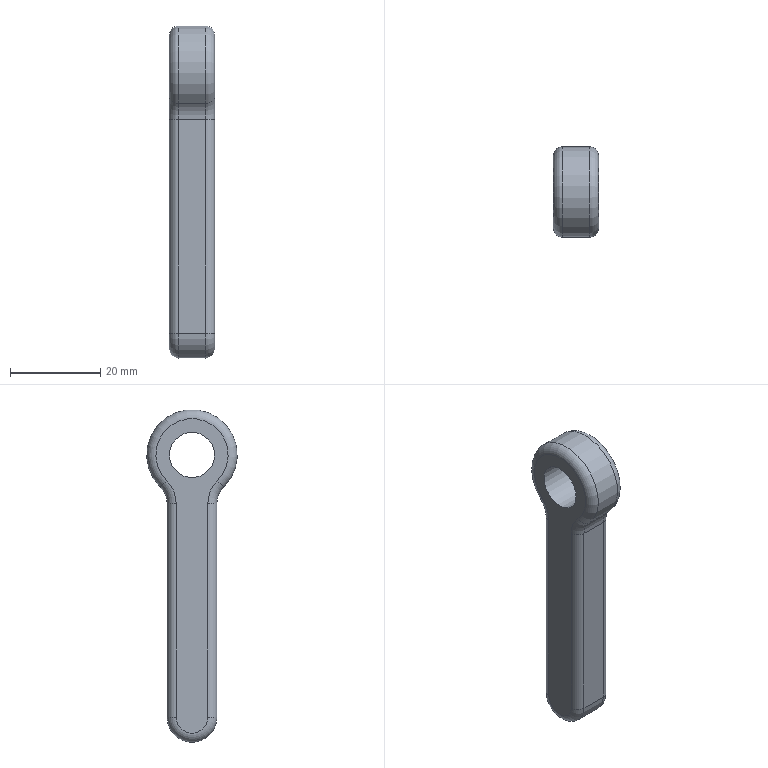Part | NX | features DATUM_CSYS 2, BLEND 1, EXTRUDE 1, SKETCH 1 | 1 solid | 21 faces | box 10 x 20 x 73.5 mm | volume 7901 mm3 | cylinder 9 | torus 8 | plane 4 | commonest cylinder face diameters 4 x4 10 x3 11 x1 20 x1
STEP:
#1=CARTESIAN_POINT('',(8.,-7.,-7.141));
#2=VERTEX_POINT('',#1);
#3=CARTESIAN_POINT('',(2.,-7.,-7.141));
#4=VERTEX_POINT('',#3);
#5=CARTESIAN_POINT('',(10.,-7.,-7.141));
#6=DIRECTION('',(-1.,0.,0.));
#7=VECTOR('',#6,1000.);
#8=LINE('',#5,#7);
#9=EDGE_CURVE('',#2,#4,#8,.T.);
#10=ORIENTED_EDGE('',*,*,#9,.T.);
#11=CARTESIAN_POINT('',(2.,-5.5,-10.712));
#12=VERTEX_POINT('',#11);
#13=CARTESIAN_POINT('',(2.,-10.5,-10.712));
#14=DIRECTION('',(-1.,0.,0.));
#15=DIRECTION('',(0.,0.,1.));
#16=AXIS2_PLACEMENT_3D('',#13,#14,#15);
#17=CIRCLE('',#16,5.);
#18=EDGE_CURVE('',#4,#12,#17,.T.);
#19=ORIENTED_EDGE('',*,*,#18,.T.);
#20=CARTESIAN_POINT('',(8.,-5.5,-10.712));
#21=VERTEX_POINT('',#20);
#22=CARTESIAN_POINT('',(10.,-5.5,-10.712));
#23=DIRECTION('',(-1.,0.,0.));
#24=VECTOR('',#23,1000.);
#25=LINE('',#22,#24);
#26=EDGE_CURVE('',#21,#12,#25,.T.);
#27=ORIENTED_EDGE('',*,*,#26,.F.);
#28=CARTESIAN_POINT('',(8.,-10.5,-10.712));
#29=DIRECTION('',(-1.,0.,0.));
#30=DIRECTION('',(0.,0.,1.));
#31=AXIS2_PLACEMENT_3D('',#28,#29,#30);
#32=CIRCLE('',#31,5.);
#33=EDGE_CURVE('',#21,#2,#32,.F.);
#34=ORIENTED_EDGE('',*,*,#33,.T.);
#35=EDGE_LOOP('',(#10,#19,#27,#34));
#36=FACE_BOUND('',#35,.T.);
#37=CARTESIAN_POINT('',(10.,-10.5,-10.712));
#38=DIRECTION('',(-1.,0.,0.));
#39=DIRECTION('',(0.,0.,1.));
#40=AXIS2_PLACEMENT_3D('',#37,#38,#39);
#41=CYLINDRICAL_SURFACE('',#40,5.);
#42=ADVANCED_FACE('',(#36),#41,.F.);
#43=ORIENTED_EDGE('',*,*,#26,.T.);
#44=CARTESIAN_POINT('',(2.,-5.5,-58.));
#45=VERTEX_POINT('',#44);
#46=CARTESIAN_POINT('',(2.,-5.5,-58.));
#47=DIRECTION('',(0.,0.,-1.));
#48=VECTOR('',#47,1000.);
#49=LINE('',#46,#48);
#50=EDGE_CURVE('',#12,#45,#49,.T.);
#51=ORIENTED_EDGE('',*,*,#50,.T.);
#52=CARTESIAN_POINT('',(8.,-5.5,-58.));
#53=VERTEX_POINT('',#52);
#54=CARTESIAN_POINT('',(10.,-5.5,-58.));
#55=DIRECTION('',(-1.,0.,0.));
#56=VECTOR('',#55,1000.);
#57=LINE('',#54,#56);
#58=EDGE_CURVE('',#53,#45,#57,.T.);
#59=ORIENTED_EDGE('',*,*,#58,.F.);
#60=CARTESIAN_POINT('',(8.,-5.5,-10.712));
#61=DIRECTION('',(0.,0.,-1.));
#62=VECTOR('',#61,1000.);
#63=LINE('',#60,#62);
#64=EDGE_CURVE('',#53,#21,#63,.F.);
#65=ORIENTED_EDGE('',*,*,#64,.T.);
#66=EDGE_LOOP('',(#43,#51,#59,#65));
#67=FACE_BOUND('',#66,.T.);
#68=CARTESIAN_POINT('',(10.,-5.5,-10.712));
#69=DIRECTION('',(0.,1.,0.));
#70=DIRECTION('',(0.,0.,1.));
#71=AXIS2_PLACEMENT_3D('',#68,#69,#70);
#72=PLANE('',#71);
#73=ADVANCED_FACE('',(#67),#72,.F.);
#74=ORIENTED_EDGE('',*,*,#58,.T.);
#75=CARTESIAN_POINT('',(2.,5.5,-58.));
#76=VERTEX_POINT('',#75);
#77=CARTESIAN_POINT('',(2.,0.,-58.));
#78=DIRECTION('',(-1.,0.,0.));
#79=DIRECTION('',(0.,0.,1.));
#80=AXIS2_PLACEMENT_3D('',#77,#78,#79);
#81=CIRCLE('',#80,5.5);
#82=EDGE_CURVE('',#45,#76,#81,.F.);
#83=ORIENTED_EDGE('',*,*,#82,.T.);
#84=CARTESIAN_POINT('',(8.,5.5,-58.));
#85=VERTEX_POINT('',#84);
#86=CARTESIAN_POINT('',(10.,5.5,-58.));
#87=DIRECTION('',(-1.,0.,0.));
#88=VECTOR('',#87,1000.);
#89=LINE('',#86,#88);
#90=EDGE_CURVE('',#85,#76,#89,.T.);
#91=ORIENTED_EDGE('',*,*,#90,.F.);
#92=CARTESIAN_POINT('',(8.,0.,-58.));
#93=DIRECTION('',(-1.,0.,0.));
#94=DIRECTION('',(0.,0.,1.));
#95=AXIS2_PLACEMENT_3D('',#92,#93,#94);
#96=CIRCLE('',#95,5.5);
#97=EDGE_CURVE('',#85,#53,#96,.T.);
#98=ORIENTED_EDGE('',*,*,#97,.T.);
#99=EDGE_LOOP('',(#74,#83,#91,#98));
#100=FACE_BOUND('',#99,.T.);
#101=CARTESIAN_POINT('',(10.,0.,-58.));
#102=DIRECTION('',(-1.,0.,0.));
#103=DIRECTION('',(0.,0.,1.));
#104=AXIS2_PLACEMENT_3D('',#101,#102,#103);
#105=CYLINDRICAL_SURFACE('',#104,5.5);
#106=ADVANCED_FACE('',(#100),#105,.T.);
#107=ORIENTED_EDGE('',*,*,#90,.T.);
#108=CARTESIAN_POINT('',(2.,5.5,-10.712));
#109=VERTEX_POINT('',#108);
#110=CARTESIAN_POINT('',(2.,5.5,-10.712));
#111=DIRECTION('',(0.,0.,1.));
#112=VECTOR('',#111,1000.);
#113=LINE('',#110,#112);
#114=EDGE_CURVE('',#76,#109,#113,.T.);
#115=ORIENTED_EDGE('',*,*,#114,.T.);
#116=CARTESIAN_POINT('',(8.,5.5,-10.712));
#117=VERTEX_POINT('',#116);
#118=CARTESIAN_POINT('',(10.,5.5,-10.712));
#119=DIRECTION('',(-1.,0.,0.));
#120=VECTOR('',#119,1000.);
#121=LINE('',#118,#120);
#122=EDGE_CURVE('',#117,#109,#121,.T.);
#123=ORIENTED_EDGE('',*,*,#122,.F.);
#124=CARTESIAN_POINT('',(8.,5.5,-58.));
#125=DIRECTION('',(0.,0.,1.));
#126=VECTOR('',#125,1000.);
#127=LINE('',#124,#126);
#128=EDGE_CURVE('',#117,#85,#127,.F.);
#129=ORIENTED_EDGE('',*,*,#128,.T.);
#130=EDGE_LOOP('',(#107,#115,#123,#129));
#131=FACE_BOUND('',#130,.T.);
#132=CARTESIAN_POINT('',(10.,5.5,-58.));
#133=DIRECTION('',(0.,-1.,0.));
#134=DIRECTION('',(0.,0.,-1.));
#135=AXIS2_PLACEMENT_3D('',#132,#133,#134);
#136=PLANE('',#135);
#137=ADVANCED_FACE('',(#131),#136,.F.);
#138=ORIENTED_EDGE('',*,*,#122,.T.);
#139=CARTESIAN_POINT('',(2.,7.,-7.141));
#140=VERTEX_POINT('',#139);
#141=CARTESIAN_POINT('',(2.,10.5,-10.712));
#142=DIRECTION('',(-1.,0.,0.));
#143=DIRECTION('',(0.,0.,1.));
#144=AXIS2_PLACEMENT_3D('',#141,#142,#143);
#145=CIRCLE('',#144,5.);
#146=EDGE_CURVE('',#109,#140,#145,.T.);
#147=ORIENTED_EDGE('',*,*,#146,.T.);
#148=CARTESIAN_POINT('',(8.,7.,-7.141));
#149=VERTEX_POINT('',#148);
#150=CARTESIAN_POINT('',(10.,7.,-7.141));
#151=DIRECTION('',(-1.,0.,0.));
#152=VECTOR('',#151,1000.);
#153=LINE('',#150,#152);
#154=EDGE_CURVE('',#149,#140,#153,.T.);
#155=ORIENTED_EDGE('',*,*,#154,.F.);
#156=CARTESIAN_POINT('',(8.,10.5,-10.712));
#157=DIRECTION('',(-1.,0.,0.));
#158=DIRECTION('',(0.,0.,1.));
#159=AXIS2_PLACEMENT_3D('',#156,#157,#158);
#160=CIRCLE('',#159,5.);
#161=EDGE_CURVE('',#149,#117,#160,.F.);
#162=ORIENTED_EDGE('',*,*,#161,.T.);
#163=EDGE_LOOP('',(#138,#147,#155,#162));
#164=FACE_BOUND('',#163,.T.);
#165=CARTESIAN_POINT('',(10.,10.5,-10.712));
#166=DIRECTION('',(-1.,0.,0.));
#167=DIRECTION('',(0.,0.,1.));
#168=AXIS2_PLACEMENT_3D('',#165,#166,#167);
#169=CYLINDRICAL_SURFACE('',#168,5.);
#170=ADVANCED_FACE('',(#164),#169,.F.);
#171=ORIENTED_EDGE('',*,*,#154,.T.);
#172=CARTESIAN_POINT('',(2.,0.,0.));
#173=DIRECTION('',(-1.,0.,0.));
#174=DIRECTION('',(0.,0.,1.));
#175=AXIS2_PLACEMENT_3D('',#172,#173,#174);
#176=CIRCLE('',#175,10.);
#177=EDGE_CURVE('',#140,#4,#176,.F.);
#178=ORIENTED_EDGE('',*,*,#177,.T.);
#179=ORIENTED_EDGE('',*,*,#9,.F.);
#180=CARTESIAN_POINT('',(8.,0.,0.));
#181=DIRECTION('',(-1.,0.,0.));
#182=DIRECTION('',(0.,0.,1.));
#183=AXIS2_PLACEMENT_3D('',#180,#181,#182);
#184=CIRCLE('',#183,10.);
#185=EDGE_CURVE('',#2,#149,#184,.T.);
#186=ORIENTED_EDGE('',*,*,#185,.T.);
#187=EDGE_LOOP('',(#171,#178,#179,#186));
#188=FACE_BOUND('',#187,.T.);
#189=CARTESIAN_POINT('',(10.,0.,0.));
#190=DIRECTION('',(-1.,0.,0.));
#191=DIRECTION('',(0.,0.,1.));
#192=AXIS2_PLACEMENT_3D('',#189,#190,#191);
#193=CYLINDRICAL_SURFACE('',#192,10.);
#194=ADVANCED_FACE('',(#188),#193,.T.);
#195=CARTESIAN_POINT('',(10.,5.,0.));
#196=VERTEX_POINT('',#195);
#197=CARTESIAN_POINT('',(10.,0.,0.));
#198=DIRECTION('',(1.,0.,0.));
#199=DIRECTION('',(0.,1.,0.));
#200=AXIS2_PLACEMENT_3D('',#197,#198,#199);
#201=CIRCLE('',#200,5.);
#202=EDGE_CURVE('',#196,#196,#201,.T.);
#203=ORIENTED_EDGE('',*,*,#202,.T.);
#204=EDGE_LOOP('',(#203));
#205=FACE_BOUND('',#204,.T.);
#206=CARTESIAN_POINT('',(0.,5.,0.));
#207=VERTEX_POINT('',#206);
#208=CARTESIAN_POINT('',(0.,0.,0.));
#209=DIRECTION('',(1.,0.,0.));
#210=DIRECTION('',(0.,1.,0.));
#211=AXIS2_PLACEMENT_3D('',#208,#209,#210);
#212=CIRCLE('',#211,5.);
#213=EDGE_CURVE('',#207,#207,#212,.T.);
#214=ORIENTED_EDGE('',*,*,#213,.F.);
#215=EDGE_LOOP('',(#214));
#216=FACE_BOUND('',#215,.T.);
#217=CARTESIAN_POINT('',(10.,0.,0.));
#218=DIRECTION('',(-1.,0.,0.));
#219=DIRECTION('',(0.,0.,1.));
#220=AXIS2_PLACEMENT_3D('',#217,#218,#219);
#221=CYLINDRICAL_SURFACE('',#220,5.);
#222=ADVANCED_FACE('',(#205,#216),#221,.F.);
#223=CARTESIAN_POINT('',(10.,3.5,-58.));
#224=VERTEX_POINT('',#223);
#225=CARTESIAN_POINT('',(10.,3.5,-10.712));
#226=VERTEX_POINT('',#225);
#227=CARTESIAN_POINT('',(10.,3.5,-10.712));
#228=DIRECTION('',(0.,0.,1.));
#229=VECTOR('',#228,1000.);
#230=LINE('',#227,#229);
#231=EDGE_CURVE('',#224,#226,#230,.T.);
#232=ORIENTED_EDGE('',*,*,#231,.T.);
#233=CARTESIAN_POINT('',(10.,5.6,-5.713));
#234=VERTEX_POINT('',#233);
#235=CARTESIAN_POINT('',(10.,10.5,-10.712));
#236=DIRECTION('',(-1.,0.,0.));
#237=DIRECTION('',(0.,0.,1.));
#238=AXIS2_PLACEMENT_3D('',#235,#236,#237);
#239=CIRCLE('',#238,7.);
#240=EDGE_CURVE('',#226,#234,#239,.T.);
#241=ORIENTED_EDGE('',*,*,#240,.T.);
#242=CARTESIAN_POINT('',(10.,-5.6,-5.713));
#243=VERTEX_POINT('',#242);
#244=CARTESIAN_POINT('',(10.,0.,0.));
#245=DIRECTION('',(-1.,0.,0.));
#246=DIRECTION('',(0.,0.,1.));
#247=AXIS2_PLACEMENT_3D('',#244,#245,#246);
#248=CIRCLE('',#247,8.);
#249=EDGE_CURVE('',#234,#243,#248,.F.);
#250=ORIENTED_EDGE('',*,*,#249,.T.);
#251=CARTESIAN_POINT('',(10.,-3.5,-10.712));
#252=VERTEX_POINT('',#251);
#253=CARTESIAN_POINT('',(10.,-10.5,-10.712));
#254=DIRECTION('',(-1.,0.,0.));
#255=DIRECTION('',(0.,0.,1.));
#256=AXIS2_PLACEMENT_3D('',#253,#254,#255);
#257=CIRCLE('',#256,7.);
#258=EDGE_CURVE('',#243,#252,#257,.T.);
#259=ORIENTED_EDGE('',*,*,#258,.T.);
#260=CARTESIAN_POINT('',(10.,-3.5,-58.));
#261=VERTEX_POINT('',#260);
#262=CARTESIAN_POINT('',(10.,-3.5,-10.712));
#263=DIRECTION('',(0.,0.,-1.));
#264=VECTOR('',#263,1000.);
#265=LINE('',#262,#264);
#266=EDGE_CURVE('',#252,#261,#265,.T.);
#267=ORIENTED_EDGE('',*,*,#266,.T.);
#268=CARTESIAN_POINT('',(10.,0.,-58.));
#269=DIRECTION('',(-1.,0.,0.));
#270=DIRECTION('',(0.,0.,1.));
#271=AXIS2_PLACEMENT_3D('',#268,#269,#270);
#272=CIRCLE('',#271,3.5);
#273=EDGE_CURVE('',#261,#224,#272,.F.);
#274=ORIENTED_EDGE('',*,*,#273,.T.);
#275=EDGE_LOOP('',(#232,#241,#250,#259,#267,#274));
#276=FACE_BOUND('',#275,.T.);
#277=ORIENTED_EDGE('',*,*,#202,.F.);
#278=EDGE_LOOP('',(#277));
#279=FACE_BOUND('',#278,.T.);
#280=CARTESIAN_POINT('',(10.,-10.5,-10.712));
#281=DIRECTION('',(-1.,0.,0.));
#282=DIRECTION('',(0.,0.,1.));
#283=AXIS2_PLACEMENT_3D('',#280,#281,#282);
#284=PLANE('',#283);
#285=ADVANCED_FACE('',(#276,#279),#284,.F.);
#286=CARTESIAN_POINT('',(0.,3.5,-58.));
#287=VERTEX_POINT('',#286);
#288=CARTESIAN_POINT('',(0.,-3.5,-58.));
#289=VERTEX_POINT('',#288);
#290=CARTESIAN_POINT('',(0.,0.,-58.));
#291=DIRECTION('',(-1.,0.,0.));
#292=DIRECTION('',(0.,0.,1.));
#293=AXIS2_PLACEMENT_3D('',#290,#291,#292);
#294=CIRCLE('',#293,3.5);
#295=EDGE_CURVE('',#287,#289,#294,.T.);
#296=ORIENTED_EDGE('',*,*,#295,.T.);
#297=CARTESIAN_POINT('',(0.,-3.5,-10.712));
#298=VERTEX_POINT('',#297);
#299=CARTESIAN_POINT('',(0.,-3.5,-10.712));
#300=DIRECTION('',(0.,0.,-1.));
#301=VECTOR('',#300,1000.);
#302=LINE('',#299,#301);
#303=EDGE_CURVE('',#289,#298,#302,.F.);
#304=ORIENTED_EDGE('',*,*,#303,.T.);
#305=CARTESIAN_POINT('',(0.,-5.6,-5.713));
#306=VERTEX_POINT('',#305);
#307=CARTESIAN_POINT('',(0.,-10.5,-10.712));
#308=DIRECTION('',(-1.,0.,0.));
#309=DIRECTION('',(0.,0.,1.));
#310=AXIS2_PLACEMENT_3D('',#307,#308,#309);
#311=CIRCLE('',#310,7.);
#312=EDGE_CURVE('',#298,#306,#311,.F.);
#313=ORIENTED_EDGE('',*,*,#312,.T.);
#314=CARTESIAN_POINT('',(0.,5.6,-5.713));
#315=VERTEX_POINT('',#314);
#316=CARTESIAN_POINT('',(0.,0.,0.));
#317=DIRECTION('',(-1.,0.,0.));
#318=DIRECTION('',(0.,0.,1.));
#319=AXIS2_PLACEMENT_3D('',#316,#317,#318);
#320=CIRCLE('',#319,8.);
#321=EDGE_CURVE('',#306,#315,#320,.T.);
#322=ORIENTED_EDGE('',*,*,#321,.T.);
#323=CARTESIAN_POINT('',(0.,3.5,-10.712));
#324=VERTEX_POINT('',#323);
#325=CARTESIAN_POINT('',(0.,10.5,-10.712));
#326=DIRECTION('',(-1.,0.,0.));
#327=DIRECTION('',(0.,0.,1.));
#328=AXIS2_PLACEMENT_3D('',#325,#326,#327);
#329=CIRCLE('',#328,7.);
#330=EDGE_CURVE('',#315,#324,#329,.F.);
#331=ORIENTED_EDGE('',*,*,#330,.T.);
#332=CARTESIAN_POINT('',(0.,3.5,-58.));
#333=DIRECTION('',(0.,0.,1.));
#334=VECTOR('',#333,1000.);
#335=LINE('',#332,#334);
#336=EDGE_CURVE('',#324,#287,#335,.F.);
#337=ORIENTED_EDGE('',*,*,#336,.T.);
#338=EDGE_LOOP('',(#296,#304,#313,#322,#331,#337));
#339=FACE_BOUND('',#338,.T.);
#340=ORIENTED_EDGE('',*,*,#213,.T.);
#341=EDGE_LOOP('',(#340));
#342=FACE_BOUND('',#341,.T.);
#343=CARTESIAN_POINT('',(0.,-10.5,-10.712));
#344=DIRECTION('',(-1.,0.,0.));
#345=DIRECTION('',(0.,0.,1.));
#346=AXIS2_PLACEMENT_3D('',#343,#344,#345);
#347=PLANE('',#346);
#348=ADVANCED_FACE('',(#339,#342),#347,.T.);
#349=CARTESIAN_POINT('',(2.,3.5,-10.712));
#350=DIRECTION('',(0.,0.,-1.));
#351=DIRECTION('',(-1.,0.,0.));
#352=AXIS2_PLACEMENT_3D('',#349,#350,#351);
#353=CIRCLE('',#352,2.);
#354=EDGE_CURVE('',#324,#109,#353,.T.);
#355=ORIENTED_EDGE('',*,*,#354,.F.);
#356=ORIENTED_EDGE('',*,*,#330,.F.);
#357=CARTESIAN_POINT('',(2.,5.6,-5.713));
#358=DIRECTION('',(0.,0.7141,0.7));
#359=DIRECTION('',(0.,-0.7,0.7141));
#360=AXIS2_PLACEMENT_3D('',#357,#358,#359);
#361=CIRCLE('',#360,2.);
#362=EDGE_CURVE('',#140,#315,#361,.T.);
#363=ORIENTED_EDGE('',*,*,#362,.F.);
#364=ORIENTED_EDGE('',*,*,#146,.F.);
#365=EDGE_LOOP('',(#355,#356,#363,#364));
#366=FACE_BOUND('',#365,.T.);
#367=CARTESIAN_POINT('',(2.,10.5,-10.712));
#368=DIRECTION('',(-1.,0.,0.));
#369=DIRECTION('',(0.,0.,1.));
#370=AXIS2_PLACEMENT_3D('',#367,#368,#369);
#371=TOROIDAL_SURFACE('',#370,7.,2.);
#372=ADVANCED_FACE('',(#366),#371,.T.);
#373=ORIENTED_EDGE('',*,*,#362,.T.);
#374=ORIENTED_EDGE('',*,*,#321,.F.);
#375=CARTESIAN_POINT('',(2.,-5.6,-5.713));
#376=DIRECTION('',(0.,0.7141,-0.7));
#377=DIRECTION('',(0.,0.7,0.7141));
#378=AXIS2_PLACEMENT_3D('',#375,#376,#377);
#379=CIRCLE('',#378,2.);
#380=EDGE_CURVE('',#4,#306,#379,.T.);
#381=ORIENTED_EDGE('',*,*,#380,.F.);
#382=ORIENTED_EDGE('',*,*,#177,.F.);
#383=EDGE_LOOP('',(#373,#374,#381,#382));
#384=FACE_BOUND('',#383,.T.);
#385=CARTESIAN_POINT('',(2.,0.,0.));
#386=DIRECTION('',(-1.,0.,0.));
#387=DIRECTION('',(0.,0.,1.));
#388=AXIS2_PLACEMENT_3D('',#385,#386,#387);
#389=TOROIDAL_SURFACE('',#388,8.,2.);
#390=ADVANCED_FACE('',(#384),#389,.T.);
#391=ORIENTED_EDGE('',*,*,#354,.T.);
#392=ORIENTED_EDGE('',*,*,#114,.F.);
#393=CARTESIAN_POINT('',(2.,3.5,-58.));
#394=DIRECTION('',(0.,0.,-1.));
#395=DIRECTION('',(-1.,0.,0.));
#396=AXIS2_PLACEMENT_3D('',#393,#394,#395);
#397=CIRCLE('',#396,2.);
#398=EDGE_CURVE('',#287,#76,#397,.T.);
#399=ORIENTED_EDGE('',*,*,#398,.F.);
#400=ORIENTED_EDGE('',*,*,#336,.F.);
#401=EDGE_LOOP('',(#391,#392,#399,#400));
#402=FACE_BOUND('',#401,.T.);
#403=CARTESIAN_POINT('',(2.,3.5,-58.));
#404=DIRECTION('',(0.,0.,-1.));
#405=DIRECTION('',(0.,1.,0.));
#406=AXIS2_PLACEMENT_3D('',#403,#404,#405);
#407=CYLINDRICAL_SURFACE('',#406,2.);
#408=ADVANCED_FACE('',(#402),#407,.T.);
#409=ORIENTED_EDGE('',*,*,#380,.T.);
#410=ORIENTED_EDGE('',*,*,#312,.F.);
#411=CARTESIAN_POINT('',(2.,-3.5,-10.712));
#412=DIRECTION('',(0.,0.,-1.));
#413=DIRECTION('',(-1.,0.,0.));
#414=AXIS2_PLACEMENT_3D('',#411,#412,#413);
#415=CIRCLE('',#414,2.);
#416=EDGE_CURVE('',#12,#298,#415,.T.);
#417=ORIENTED_EDGE('',*,*,#416,.F.);
#418=ORIENTED_EDGE('',*,*,#18,.F.);
#419=EDGE_LOOP('',(#409,#410,#417,#418));
#420=FACE_BOUND('',#419,.T.);
#421=CARTESIAN_POINT('',(2.,-10.5,-10.712));
#422=DIRECTION('',(-1.,0.,0.));
#423=DIRECTION('',(0.,0.,1.));
#424=AXIS2_PLACEMENT_3D('',#421,#422,#423);
#425=TOROIDAL_SURFACE('',#424,7.,2.);
#426=ADVANCED_FACE('',(#420),#425,.T.);
#427=ORIENTED_EDGE('',*,*,#398,.T.);
#428=ORIENTED_EDGE('',*,*,#82,.F.);
#429=CARTESIAN_POINT('',(2.,-3.5,-58.));
#430=DIRECTION('',(0.,0.,1.));
#431=DIRECTION('',(1.,0.,0.));
#432=AXIS2_PLACEMENT_3D('',#429,#430,#431);
#433=CIRCLE('',#432,2.);
#434=EDGE_CURVE('',#289,#45,#433,.T.);
#435=ORIENTED_EDGE('',*,*,#434,.F.);
#436=ORIENTED_EDGE('',*,*,#295,.F.);
#437=EDGE_LOOP('',(#427,#428,#435,#436));
#438=FACE_BOUND('',#437,.T.);
#439=CARTESIAN_POINT('',(2.,0.,-58.));
#440=DIRECTION('',(-1.,0.,0.));
#441=DIRECTION('',(0.,0.,1.));
#442=AXIS2_PLACEMENT_3D('',#439,#440,#441);
#443=TOROIDAL_SURFACE('',#442,3.5,2.);
#444=ADVANCED_FACE('',(#438),#443,.T.);
#445=ORIENTED_EDGE('',*,*,#416,.T.);
#446=ORIENTED_EDGE('',*,*,#303,.F.);
#447=ORIENTED_EDGE('',*,*,#434,.T.);
#448=ORIENTED_EDGE('',*,*,#50,.F.);
#449=EDGE_LOOP('',(#445,#446,#447,#448));
#450=FACE_BOUND('',#449,.T.);
#451=CARTESIAN_POINT('',(2.,-3.5,-10.712));
#452=DIRECTION('',(0.,0.,1.));
#453=DIRECTION('',(0.,-1.,0.));
#454=AXIS2_PLACEMENT_3D('',#451,#452,#453);
#455=CYLINDRICAL_SURFACE('',#454,2.);
#456=ADVANCED_FACE('',(#450),#455,.T.);
#457=CARTESIAN_POINT('',(8.,-3.5,-10.712));
#458=DIRECTION('',(0.,0.,1.));
#459=DIRECTION('',(1.,0.,0.));
#460=AXIS2_PLACEMENT_3D('',#457,#458,#459);
#461=CIRCLE('',#460,2.);
#462=EDGE_CURVE('',#21,#252,#461,.T.);
#463=ORIENTED_EDGE('',*,*,#462,.F.);
#464=ORIENTED_EDGE('',*,*,#64,.F.);
#465=CARTESIAN_POINT('',(8.,-3.5,-58.));
#466=DIRECTION('',(0.,0.,-1.));
#467=DIRECTION('',(-1.,0.,0.));
#468=AXIS2_PLACEMENT_3D('',#465,#466,#467);
#469=CIRCLE('',#468,2.);
#470=EDGE_CURVE('',#261,#53,#469,.T.);
#471=ORIENTED_EDGE('',*,*,#470,.F.);
#472=ORIENTED_EDGE('',*,*,#266,.F.);
#473=EDGE_LOOP('',(#463,#464,#471,#472));
#474=FACE_BOUND('',#473,.T.);
#475=CARTESIAN_POINT('',(8.,-3.5,-10.712));
#476=DIRECTION('',(0.,0.,-1.));
#477=DIRECTION('',(0.,1.,0.));
#478=AXIS2_PLACEMENT_3D('',#475,#476,#477);
#479=CYLINDRICAL_SURFACE('',#478,2.);
#480=ADVANCED_FACE('',(#474),#479,.T.);
#481=ORIENTED_EDGE('',*,*,#470,.T.);
#482=ORIENTED_EDGE('',*,*,#97,.F.);
#483=CARTESIAN_POINT('',(8.,3.5,-58.));
#484=DIRECTION('',(0.,0.,1.));
#485=DIRECTION('',(1.,0.,0.));
#486=AXIS2_PLACEMENT_3D('',#483,#484,#485);
#487=CIRCLE('',#486,2.);
#488=EDGE_CURVE('',#224,#85,#487,.T.);
#489=ORIENTED_EDGE('',*,*,#488,.F.);
#490=ORIENTED_EDGE('',*,*,#273,.F.);
#491=EDGE_LOOP('',(#481,#482,#489,#490));
#492=FACE_BOUND('',#491,.T.);
#493=CARTESIAN_POINT('',(8.,0.,-58.));
#494=DIRECTION('',(-1.,0.,0.));
#495=DIRECTION('',(0.,0.,1.));
#496=AXIS2_PLACEMENT_3D('',#493,#494,#495);
#497=TOROIDAL_SURFACE('',#496,3.5,2.);
#498=ADVANCED_FACE('',(#492),#497,.T.);
#499=ORIENTED_EDGE('',*,*,#462,.T.);
#500=ORIENTED_EDGE('',*,*,#258,.F.);
#501=CARTESIAN_POINT('',(8.,-5.6,-5.713));
#502=DIRECTION('',(0.,-0.7141,0.7));
#503=DIRECTION('',(0.,-0.7,-0.7141));
#504=AXIS2_PLACEMENT_3D('',#501,#502,#503);
#505=CIRCLE('',#504,2.);
#506=EDGE_CURVE('',#2,#243,#505,.T.);
#507=ORIENTED_EDGE('',*,*,#506,.F.);
#508=ORIENTED_EDGE('',*,*,#33,.F.);
#509=EDGE_LOOP('',(#499,#500,#507,#508));
#510=FACE_BOUND('',#509,.T.);
#511=CARTESIAN_POINT('',(8.,-10.5,-10.712));
#512=DIRECTION('',(-1.,0.,0.));
#513=DIRECTION('',(0.,0.,1.));
#514=AXIS2_PLACEMENT_3D('',#511,#512,#513);
#515=TOROIDAL_SURFACE('',#514,7.,2.);
#516=ADVANCED_FACE('',(#510),#515,.T.);
#517=ORIENTED_EDGE('',*,*,#488,.T.);
#518=ORIENTED_EDGE('',*,*,#128,.F.);
#519=CARTESIAN_POINT('',(8.,3.5,-10.712));
#520=DIRECTION('',(0.,0.,1.));
#521=DIRECTION('',(1.,0.,0.));
#522=AXIS2_PLACEMENT_3D('',#519,#520,#521);
#523=CIRCLE('',#522,2.);
#524=EDGE_CURVE('',#226,#117,#523,.T.);
#525=ORIENTED_EDGE('',*,*,#524,.F.);
#526=ORIENTED_EDGE('',*,*,#231,.F.);
#527=EDGE_LOOP('',(#517,#518,#525,#526));
#528=FACE_BOUND('',#527,.T.);
#529=CARTESIAN_POINT('',(8.,3.5,-10.712));
#530=DIRECTION('',(0.,0.,1.));
#531=DIRECTION('',(0.,-1.,0.));
#532=AXIS2_PLACEMENT_3D('',#529,#530,#531);
#533=CYLINDRICAL_SURFACE('',#532,2.);
#534=ADVANCED_FACE('',(#528),#533,.T.);
#535=ORIENTED_EDGE('',*,*,#506,.T.);
#536=ORIENTED_EDGE('',*,*,#249,.F.);
#537=CARTESIAN_POINT('',(8.,5.6,-5.713));
#538=DIRECTION('',(0.,-0.7141,-0.7));
#539=DIRECTION('',(0.,0.7,-0.7141));
#540=AXIS2_PLACEMENT_3D('',#537,#538,#539);
#541=CIRCLE('',#540,2.);
#542=EDGE_CURVE('',#149,#234,#541,.T.);
#543=ORIENTED_EDGE('',*,*,#542,.F.);
#544=ORIENTED_EDGE('',*,*,#185,.F.);
#545=EDGE_LOOP('',(#535,#536,#543,#544));
#546=FACE_BOUND('',#545,.T.);
#547=CARTESIAN_POINT('',(8.,0.,0.));
#548=DIRECTION('',(-1.,0.,0.));
#549=DIRECTION('',(0.,0.,1.));
#550=AXIS2_PLACEMENT_3D('',#547,#548,#549);
#551=TOROIDAL_SURFACE('',#550,8.,2.);
#552=ADVANCED_FACE('',(#546),#551,.T.);
#553=ORIENTED_EDGE('',*,*,#524,.T.);
#554=ORIENTED_EDGE('',*,*,#161,.F.);
#555=ORIENTED_EDGE('',*,*,#542,.T.);
#556=ORIENTED_EDGE('',*,*,#240,.F.);
#557=EDGE_LOOP('',(#553,#554,#555,#556));
#558=FACE_BOUND('',#557,.T.);
#559=CARTESIAN_POINT('',(8.,10.5,-10.712));
#560=DIRECTION('',(-1.,0.,0.));
#561=DIRECTION('',(0.,0.,1.));
#562=AXIS2_PLACEMENT_3D('',#559,#560,#561);
#563=TOROIDAL_SURFACE('',#562,7.,2.);
#564=ADVANCED_FACE('',(#558),#563,.T.);
#565=CLOSED_SHELL('',(#42,#73,#106,#137,#170,#194,#222,#285,#348,#372,#390,#408,#426,#444,#456,#480,#498,#516,#534,#552,#564));
#566=MANIFOLD_SOLID_BREP('',#565);
#567=(LENGTH_UNIT()NAMED_UNIT(*)SI_UNIT(.MILLI.,.METRE.));
#568=UNCERTAINTY_MEASURE_WITH_UNIT(LENGTH_MEASURE(0.00001),#567,'','');
#569=(NAMED_UNIT(*)PLANE_ANGLE_UNIT()SI_UNIT($,.RADIAN.));
#570=(NAMED_UNIT(*)SI_UNIT($,.STERADIAN.)SOLID_ANGLE_UNIT());
#571=(GEOMETRIC_REPRESENTATION_CONTEXT(3)GLOBAL_UNCERTAINTY_ASSIGNED_CONTEXT((#568))GLOBAL_UNIT_ASSIGNED_CONTEXT((#567,#569,#570))REPRESENTATION_CONTEXT('',''));
#572=ADVANCED_BREP_SHAPE_REPRESENTATION('',(#566),#571);